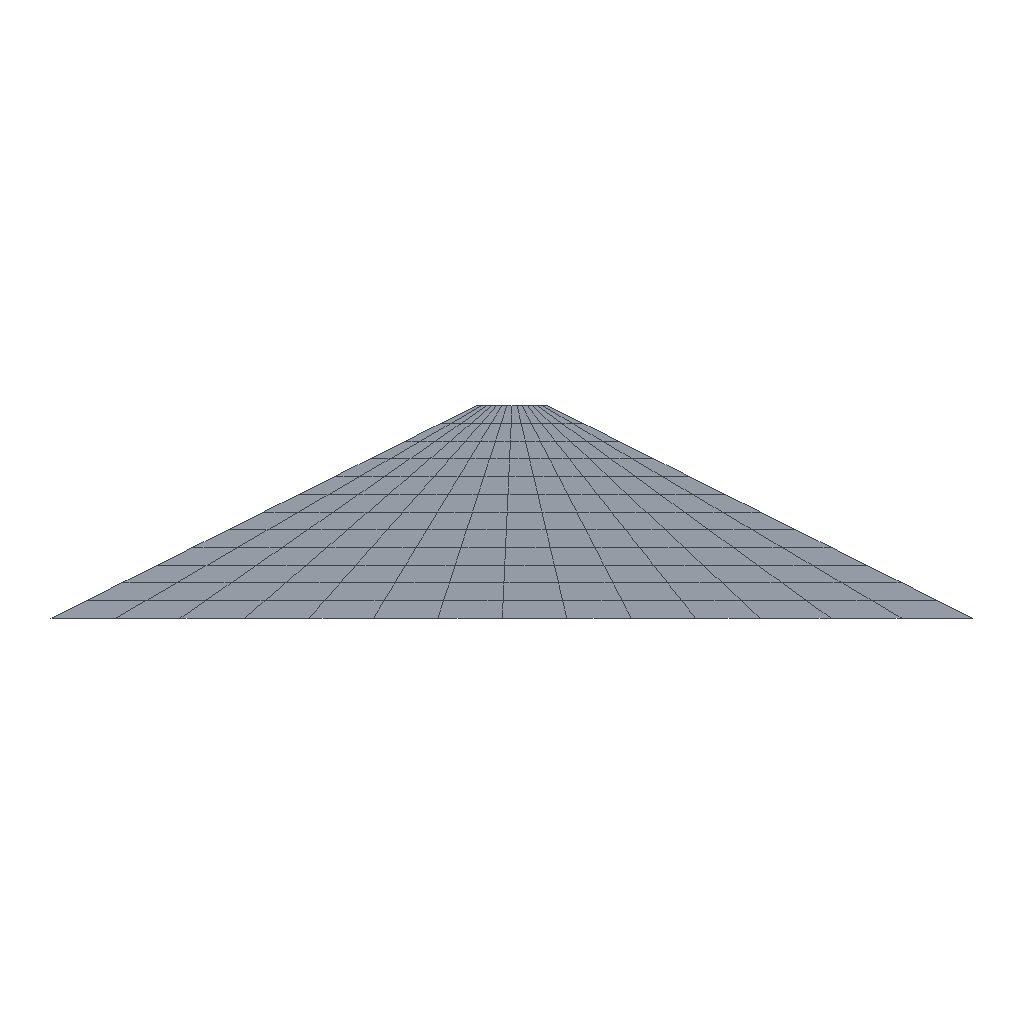Simulation study | abaqus
Set-up summary:
category,name,step,type,value,unit,region
solver,abaqus,,Abaqus/CAE 2024
units,unstated,,unstated,E=10000 density=2 (no match)
analysis,Step-1,,soils,time_period=10
mesh,nodes,,,195
mesh,elements,,,168
element_type,CPE4P,,,168
material,soil,,E,10000
material,soil,,nu,0.3
material,soil,,density,2
section,soil,,solid section,,,_PickedSet21
load,sat,initial,initial condition saturation
load,void,initial,initial condition ratio
load,Load-1,Step-1,gravity,10,,_PickedSet6
bc,BC-1,Step-1,fixed,"[dofs=x,y n=2]",,_PickedSet4
bc,BC-2,Step-1,displacement,100 [dofs=8],,dam-1.1
bc,BC-2,Step-1,displacement,90 [dofs=8],,dam-1.16
bc,BC-2,Step-1,displacement,80 [dofs=8],,dam-1.31
bc,BC-2,Step-1,displacement,70 [dofs=8],,dam-1.46
bc,BC-2,Step-1,displacement,60 [dofs=8],,dam-1.61
bc,BC-2,Step-1,displacement,50 [dofs=8],,dam-1.76
bc,BC-2,Step-1,displacement,40 [dofs=8],,dam-1.91
bc,BC-2,Step-1,displacement,30 [dofs=8],,dam-1.106
bc,BC-2,Step-1,displacement,20 [dofs=8],,dam-1.121
bc,BC-2,Step-1,displacement,10 [dofs=8],,dam-1.136
bc,BC-2,Step-1,fixed,[dofs=8],,dam-1.151
Abaqus input file, long lists of numbers shortened:
*Heading
** Job name: deck Model name: Model-1
** Generated by: Abaqus/CAE 2024
*Preprint, echo=NO, model=NO, history=NO, contact=NO
**
** PARTS
**
*Part, name=dam
*Node
      1,           0.,           0.
      2,   3.636,           0.
** (193 more lines like these left out)
*Element, type=CPE4P
  1,   1,   2,  17,  16
  2,   2,   3,  18,  17
** (166 more lines like these left out)
*Nset, nset=dam, generate
   1,  195,    1
*Elset, elset=dam, generate
   1,  168,    1
*Nset, nset=_PickedSet21, internal, generate
   1,  195,    1
*Elset, elset=_PickedSet21, internal, generate
   1,  168,    1
*Elset, elset=_Fup_S4, internal, generate
   1,  127,   14
*Surface, type=ELEMENT, name=Fup
_Fup_S4, S4
*Elset, elset=_Fbot_S1, internal, generate
 12,  14,   1
*Surface, type=ELEMENT, name=Fbot
_Fbot_S1, S1
*Elset, elset=_Fdown_S2, internal, generate
  14,  168,   14
*Surface, type=ELEMENT, name=Fdown
_Fdown_S2, S2
** Section: soil
*Solid Section, elset=_PickedSet21, material=soil
1.,
*End Part
**
**
** ASSEMBLY
**
*Assembly, name=Assembly
**
*Instance, name=dam-1, part=dam
*End Instance
**
*Nset, nset=_PickedSet4, internal, instance=dam-1, generate
   1,  195,    1
*Elset, elset=_PickedSet4, internal, instance=dam-1, generate
   1,  168,    1
*Nset, nset=_PickedSet6, internal, instance=dam-1, generate
   1,  195,    1
*Elset, elset=_PickedSet6, internal, instance=dam-1, generate
   1,  168,    1
*Nset, nset=_PickedSet7, internal, instance=dam-1, generate
   1,  151,   15
*Elset, elset=_PickedSet7, internal, instance=dam-1, generate
   1,  127,   14
*Nset, nset=_PickedSet8, internal, instance=dam-1, generate
   1,  195,    1
*Elset, elset=_PickedSet8, internal, instance=dam-1, generate
   1,  168,    1
*Nset, nset=_PickedSet9, internal, instance=dam-1, generate
   1,  195,    1
*Elset, elset=_PickedSet9, internal, instance=dam-1, generate
   1,  168,    1
*Nset, nset=_PickedSet7_PP_, internal, instance=dam-1, generate
   1,  151,   15
*End Assembly
**
** MATERIALS
**
*Material, name=soil
*Density
2.,
*Elastic
10000., 0.3
*Permeability, specific=10.
 1e-07,0.
*Permeability, Type=SATURATION
     1e-05, 0.02154
    0.0001, 0.04642
     0.001,       0.1
 0.07244,  0.4169
  0.9703,      0.99
        1.,        1.
*Sorption
-200., 0.02154
-150., 0.04642
-100.,       0.1
 -50.,  0.4169
   0.,        1.
**
** PREDEFINED FIELDS
**
** Name: sat   Type: Saturation
*Initial Conditions, type=SATURATION
_PickedSet9, 1.
** Name: void   Type: Void ratio
*Initial Conditions, TYPE=RATIO
_PickedSet8, 1.
** ----------------------------------------------------------------
**
** STEP: Step-1
**
*Step, name=Step-1, nlgeom=NO
*Soils, utol=1.0, creep=none
1., 10., 0.0001, 10.,
*sflow
dam-1.fbot,qd,0.1
dam-1.fdown,qd,0.1
**
** BOUNDARY CONDITIONS
**
** Name: BC-1 Type: Displacement/Rotation
*Boundary
_PickedSet4, 1, 1
_PickedSet4, 2, 2
** Name: BC-2 Type: Pore pressure Using Analytical Field: pore
*Boundary
dam-1.1, 8, 8, 100.
dam-1.16, 8, 8, 90.
dam-1.31, 8, 8, 80.
dam-1.46, 8, 8, 70.
dam-1.61, 8, 8, 60.
dam-1.76, 8, 8, 50.
dam-1.91, 8, 8, 40.
dam-1.106, 8, 8, 30.
dam-1.121, 8, 8, 20.
dam-1.136, 8, 8, 10.
dam-1.151, 8, 8, 0.
**
** LOADS
**
** Name: Load-1   Type: Gravity
*Dload
_PickedSet6, GRAV, 10., 0., -1.
**
** OUTPUT REQUESTS
**
*Restart, write, frequency=0
*Print, solve=NO
**
** FIELD OUTPUT: F-Output-1
**
*Output, field
*Node Output
CF, POR, RF, RVF, U
*Element Output, directions=YES
FLVEL, LE, S, SAT, VOIDR
*Contact Output
PFL, PFLA, PTL, PTLA
**
** HISTORY OUTPUT: H-Output-1
**
*Output, history, variable=PRESELECT
*End Step
Results summary:
result,odb.job_status,,,JOB_STATUS_COMPLETED_SUCCESSFULLY,"consistent, unstated (Abaqus has no unit system)"
result,steps[0].procedure,Step-1,,*SOILS,"consistent, unstated (Abaqus has no unit system)"
result,steps[0].time_period,Step-1,,10,"consistent, unstated (Abaqus has no unit system)"
result,steps[0].n_frames,Step-1,,7,"consistent, unstated (Abaqus has no unit system)"
result,steps[0].last_frame.id,Step-1,,6,"consistent, unstated (Abaqus has no unit system)"
result,steps[0].last_frame.value,Step-1,,10,"consistent, unstated (Abaqus has no unit system)"
result,steps[0].last_frame.description,Step-1,,Increment      6: Step Time =    10.00,"consistent, unstated (Abaqus has no unit system)"
result,steps[0].completed,Step-1,,True,"consistent, unstated (Abaqus has no unit system)"
result,steps[0].max_U_magnitude,Step-1,,0,"consistent, unstated (Abaqus has no unit system)"
result,steps[0].max_S_mises,Step-1,,9.79579e-31,"consistent, unstated (Abaqus has no unit system)"
result,steps[0].RF_sum[1],Step-1,,1.81198e-05,"consistent, unstated (Abaqus has no unit system)"
result,steps[0].RF_sum[2],Step-1,,8272.06,"consistent, unstated (Abaqus has no unit system)"